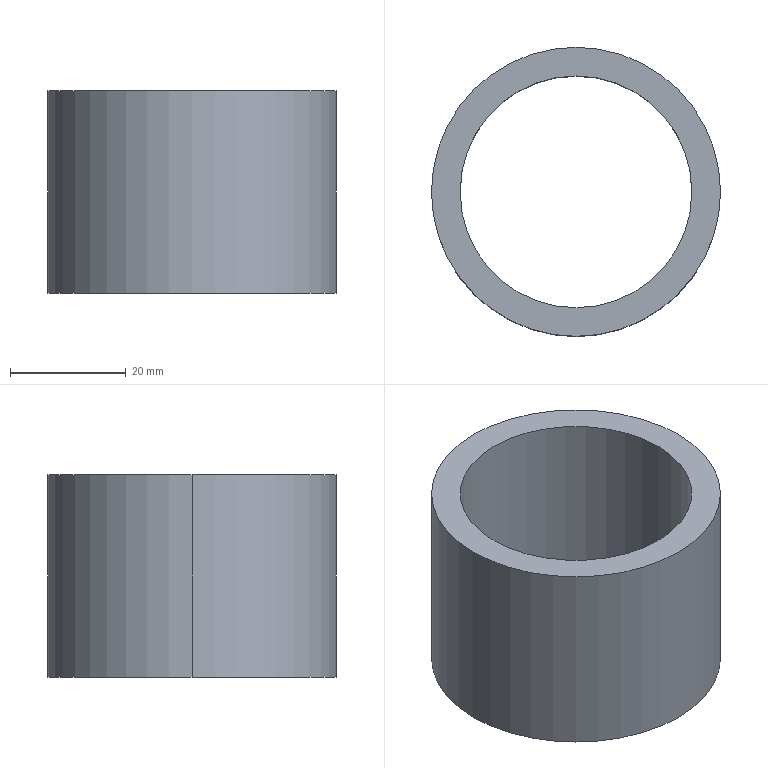Part | STEP file | LM-05-1226_default | 1 solid | 6 faces | box 50 x 50 x 35 mm | volume 24520 mm3 | cylinder 4 | plane 2 | commonest cylinder face diameters 40.1 x2 50 x2
STEP:
#1=CARTESIAN_POINT('',(0.,0.,0.));
#2=DIRECTION('',(0.,0.,1.));
#3=DIRECTION('',(1.,0.,0.));
#4=AXIS2_PLACEMENT_3D('',#1,#2,#3);
#5=CARTESIAN_POINT('',(-20.05,0.,17.5));
#6=VERTEX_POINT('',#5);
#7=CARTESIAN_POINT('',(-20.05,0.,-17.5));
#8=VERTEX_POINT('',#7);
#9=CARTESIAN_POINT('',(-20.05,0.,17.5));
#10=DIRECTION('',(0.,0.,-1.));
#11=VECTOR('',#10,1.);
#12=LINE('',#9,#11);
#13=CARTESIAN_POINT('',(0.,0.,17.5));
#14=DIRECTION('',(0.,0.,-1.));
#15=DIRECTION('',(-1.,0.,0.));
#16=AXIS2_PLACEMENT_3D('',#13,#14,#15);
#17=CYLINDRICAL_SURFACE('',#16,20.05);
#18=CARTESIAN_POINT('',(6.283,0.));
#19=DIRECTION('',(0.,1.));
#20=VECTOR('',#19,1.);
#21=LINE('',#18,#20);
#22=(GEOMETRIC_REPRESENTATION_CONTEXT(2)PARAMETRIC_REPRESENTATION_CONTEXT()REPRESENTATION_CONTEXT('',''));
#23=DEFINITIONAL_REPRESENTATION('',(#21),#22);
#24=PCURVE('',#17,#23);
#25=CARTESIAN_POINT('',(0.,0.,17.5));
#26=DIRECTION('',(0.,0.,-1.));
#27=DIRECTION('',(-1.,0.,0.));
#28=AXIS2_PLACEMENT_3D('',#25,#26,#27);
#29=CYLINDRICAL_SURFACE('',#28,20.05);
#30=CARTESIAN_POINT('',(0.,0.));
#31=DIRECTION('',(0.,1.));
#32=VECTOR('',#31,1.);
#33=LINE('',#30,#32);
#34=(GEOMETRIC_REPRESENTATION_CONTEXT(2)PARAMETRIC_REPRESENTATION_CONTEXT()REPRESENTATION_CONTEXT('',''));
#35=DEFINITIONAL_REPRESENTATION('',(#33),#34);
#36=PCURVE('',#29,#35);
#37=SURFACE_CURVE('',#12,(#24,#36),.PCURVE_S1.);
#38=EDGE_CURVE('',#6,#8,#37,.T.);
#39=ORIENTED_EDGE('',*,*,#38,.T.);
#40=CARTESIAN_POINT('',(20.05,0.,-17.5));
#41=VERTEX_POINT('',#40);
#42=CARTESIAN_POINT('',(0.,0.,-17.5));
#43=DIRECTION('',(0.,0.,1.));
#44=DIRECTION('',(1.,0.,0.));
#45=AXIS2_PLACEMENT_3D('',#42,#43,#44);
#46=CIRCLE('',#45,20.05);
#47=CARTESIAN_POINT('',(9.425,35.));
#48=DIRECTION('',(-1.,0.));
#49=VECTOR('',#48,1.);
#50=LINE('',#47,#49);
#51=(GEOMETRIC_REPRESENTATION_CONTEXT(2)PARAMETRIC_REPRESENTATION_CONTEXT()REPRESENTATION_CONTEXT('',''));
#52=DEFINITIONAL_REPRESENTATION('',(#50),#51);
#53=PCURVE('',#17,#52);
#54=CARTESIAN_POINT('',(0.,0.,-17.5));
#55=DIRECTION('',(0.,0.,1.));
#56=DIRECTION('',(1.,0.,0.));
#57=AXIS2_PLACEMENT_3D('',#54,#55,#56);
#58=PLANE('',#57);
#59=CARTESIAN_POINT('',(0.,0.));
#60=DIRECTION('',(1.,0.));
#61=AXIS2_PLACEMENT_2D('',#59,#60);
#62=CIRCLE('',#61,20.05);
#63=(GEOMETRIC_REPRESENTATION_CONTEXT(2)PARAMETRIC_REPRESENTATION_CONTEXT()REPRESENTATION_CONTEXT('',''));
#64=DEFINITIONAL_REPRESENTATION('',(#62),#63);
#65=PCURVE('',#58,#64);
#66=SURFACE_CURVE('',#46,(#53,#65),.PCURVE_S1.);
#67=EDGE_CURVE('',#8,#41,#66,.T.);
#68=ORIENTED_EDGE('',*,*,#67,.T.);
#69=CARTESIAN_POINT('',(20.05,0.,17.5));
#70=VERTEX_POINT('',#69);
#71=CARTESIAN_POINT('',(20.05,0.,17.5));
#72=DIRECTION('',(0.,0.,-1.));
#73=VECTOR('',#72,1.);
#74=LINE('',#71,#73);
#75=CARTESIAN_POINT('',(3.142,0.));
#76=DIRECTION('',(0.,1.));
#77=VECTOR('',#76,1.);
#78=LINE('',#75,#77);
#79=(GEOMETRIC_REPRESENTATION_CONTEXT(2)PARAMETRIC_REPRESENTATION_CONTEXT()REPRESENTATION_CONTEXT('',''));
#80=DEFINITIONAL_REPRESENTATION('',(#78),#79);
#81=PCURVE('',#17,#80);
#82=CARTESIAN_POINT('',(3.142,0.));
#83=DIRECTION('',(0.,1.));
#84=VECTOR('',#83,1.);
#85=LINE('',#82,#84);
#86=(GEOMETRIC_REPRESENTATION_CONTEXT(2)PARAMETRIC_REPRESENTATION_CONTEXT()REPRESENTATION_CONTEXT('',''));
#87=DEFINITIONAL_REPRESENTATION('',(#85),#86);
#88=PCURVE('',#29,#87);
#89=SURFACE_CURVE('',#74,(#81,#88),.PCURVE_S1.);
#90=EDGE_CURVE('',#70,#41,#89,.T.);
#91=ORIENTED_EDGE('',*,*,#90,.F.);
#92=CARTESIAN_POINT('',(0.,0.,17.5));
#93=DIRECTION('',(0.,0.,1.));
#94=DIRECTION('',(1.,0.,0.));
#95=AXIS2_PLACEMENT_3D('',#92,#93,#94);
#96=CIRCLE('',#95,20.05);
#97=CARTESIAN_POINT('',(9.425,0.));
#98=DIRECTION('',(-1.,0.));
#99=VECTOR('',#98,1.);
#100=LINE('',#97,#99);
#101=(GEOMETRIC_REPRESENTATION_CONTEXT(2)PARAMETRIC_REPRESENTATION_CONTEXT()REPRESENTATION_CONTEXT('',''));
#102=DEFINITIONAL_REPRESENTATION('',(#100),#101);
#103=PCURVE('',#17,#102);
#104=CARTESIAN_POINT('',(0.,0.,17.5));
#105=DIRECTION('',(0.,0.,1.));
#106=DIRECTION('',(1.,0.,0.));
#107=AXIS2_PLACEMENT_3D('',#104,#105,#106);
#108=PLANE('',#107);
#109=CARTESIAN_POINT('',(0.,0.));
#110=DIRECTION('',(1.,0.));
#111=AXIS2_PLACEMENT_2D('',#109,#110);
#112=CIRCLE('',#111,20.05);
#113=(GEOMETRIC_REPRESENTATION_CONTEXT(2)PARAMETRIC_REPRESENTATION_CONTEXT()REPRESENTATION_CONTEXT('',''));
#114=DEFINITIONAL_REPRESENTATION('',(#112),#113);
#115=PCURVE('',#108,#114);
#116=SURFACE_CURVE('',#96,(#103,#115),.PCURVE_S1.);
#117=EDGE_CURVE('',#6,#70,#116,.T.);
#118=ORIENTED_EDGE('',*,*,#117,.F.);
#119=EDGE_LOOP('',(#39,#68,#91,#118));
#120=FACE_BOUND('',#119,.F.);
#121=ADVANCED_FACE('',(#120),#17,.F.);
#122=CARTESIAN_POINT('',(25.,0.,17.5));
#123=VERTEX_POINT('',#122);
#124=CARTESIAN_POINT('',(-25.,0.,17.5));
#125=VERTEX_POINT('',#124);
#126=CARTESIAN_POINT('',(0.,0.,17.5));
#127=DIRECTION('',(0.,0.,1.));
#128=DIRECTION('',(1.,0.,0.));
#129=AXIS2_PLACEMENT_3D('',#126,#127,#128);
#130=CIRCLE('',#129,25.);
#131=CARTESIAN_POINT('',(0.,0.,17.5));
#132=DIRECTION('',(0.,0.,-1.));
#133=DIRECTION('',(-1.,0.,0.));
#134=AXIS2_PLACEMENT_3D('',#131,#132,#133);
#135=CYLINDRICAL_SURFACE('',#134,25.);
#136=CARTESIAN_POINT('',(3.142,0.));
#137=DIRECTION('',(-1.,0.));
#138=VECTOR('',#137,1.);
#139=LINE('',#136,#138);
#140=(GEOMETRIC_REPRESENTATION_CONTEXT(2)PARAMETRIC_REPRESENTATION_CONTEXT()REPRESENTATION_CONTEXT('',''));
#141=DEFINITIONAL_REPRESENTATION('',(#139),#140);
#142=PCURVE('',#135,#141);
#143=CARTESIAN_POINT('',(0.,0.));
#144=DIRECTION('',(1.,0.));
#145=AXIS2_PLACEMENT_2D('',#143,#144);
#146=CIRCLE('',#145,25.);
#147=(GEOMETRIC_REPRESENTATION_CONTEXT(2)PARAMETRIC_REPRESENTATION_CONTEXT()REPRESENTATION_CONTEXT('',''));
#148=DEFINITIONAL_REPRESENTATION('',(#146),#147);
#149=PCURVE('',#108,#148);
#150=SURFACE_CURVE('',#130,(#142,#149),.PCURVE_S1.);
#151=EDGE_CURVE('',#123,#125,#150,.T.);
#152=ORIENTED_EDGE('',*,*,#151,.F.);
#153=CARTESIAN_POINT('',(25.,0.,-17.5));
#154=VERTEX_POINT('',#153);
#155=CARTESIAN_POINT('',(25.,0.,17.5));
#156=DIRECTION('',(0.,0.,-1.));
#157=VECTOR('',#156,1.);
#158=LINE('',#155,#157);
#159=CARTESIAN_POINT('',(3.142,0.));
#160=DIRECTION('',(0.,1.));
#161=VECTOR('',#160,1.);
#162=LINE('',#159,#161);
#163=(GEOMETRIC_REPRESENTATION_CONTEXT(2)PARAMETRIC_REPRESENTATION_CONTEXT()REPRESENTATION_CONTEXT('',''));
#164=DEFINITIONAL_REPRESENTATION('',(#162),#163);
#165=PCURVE('',#135,#164);
#166=CARTESIAN_POINT('',(0.,0.,17.5));
#167=DIRECTION('',(0.,0.,-1.));
#168=DIRECTION('',(-1.,0.,0.));
#169=AXIS2_PLACEMENT_3D('',#166,#167,#168);
#170=CYLINDRICAL_SURFACE('',#169,25.);
#171=CARTESIAN_POINT('',(3.142,0.));
#172=DIRECTION('',(0.,1.));
#173=VECTOR('',#172,1.);
#174=LINE('',#171,#173);
#175=(GEOMETRIC_REPRESENTATION_CONTEXT(2)PARAMETRIC_REPRESENTATION_CONTEXT()REPRESENTATION_CONTEXT('',''));
#176=DEFINITIONAL_REPRESENTATION('',(#174),#175);
#177=PCURVE('',#170,#176);
#178=SURFACE_CURVE('',#158,(#165,#177),.PCURVE_S1.);
#179=EDGE_CURVE('',#123,#154,#178,.T.);
#180=ORIENTED_EDGE('',*,*,#179,.T.);
#181=CARTESIAN_POINT('',(-25.,0.,-17.5));
#182=VERTEX_POINT('',#181);
#183=CARTESIAN_POINT('',(0.,0.,-17.5));
#184=DIRECTION('',(0.,0.,1.));
#185=DIRECTION('',(1.,0.,0.));
#186=AXIS2_PLACEMENT_3D('',#183,#184,#185);
#187=CIRCLE('',#186,25.);
#188=CARTESIAN_POINT('',(3.142,35.));
#189=DIRECTION('',(-1.,0.));
#190=VECTOR('',#189,1.);
#191=LINE('',#188,#190);
#192=(GEOMETRIC_REPRESENTATION_CONTEXT(2)PARAMETRIC_REPRESENTATION_CONTEXT()REPRESENTATION_CONTEXT('',''));
#193=DEFINITIONAL_REPRESENTATION('',(#191),#192);
#194=PCURVE('',#135,#193);
#195=CARTESIAN_POINT('',(0.,0.));
#196=DIRECTION('',(1.,0.));
#197=AXIS2_PLACEMENT_2D('',#195,#196);
#198=CIRCLE('',#197,25.);
#199=(GEOMETRIC_REPRESENTATION_CONTEXT(2)PARAMETRIC_REPRESENTATION_CONTEXT()REPRESENTATION_CONTEXT('',''));
#200=DEFINITIONAL_REPRESENTATION('',(#198),#199);
#201=PCURVE('',#58,#200);
#202=SURFACE_CURVE('',#187,(#194,#201),.PCURVE_S1.);
#203=EDGE_CURVE('',#154,#182,#202,.T.);
#204=ORIENTED_EDGE('',*,*,#203,.T.);
#205=CARTESIAN_POINT('',(-25.,0.,17.5));
#206=DIRECTION('',(0.,0.,-1.));
#207=VECTOR('',#206,1.);
#208=LINE('',#205,#207);
#209=CARTESIAN_POINT('',(0.,0.));
#210=DIRECTION('',(0.,1.));
#211=VECTOR('',#210,1.);
#212=LINE('',#209,#211);
#213=(GEOMETRIC_REPRESENTATION_CONTEXT(2)PARAMETRIC_REPRESENTATION_CONTEXT()REPRESENTATION_CONTEXT('',''));
#214=DEFINITIONAL_REPRESENTATION('',(#212),#213);
#215=PCURVE('',#135,#214);
#216=CARTESIAN_POINT('',(6.283,0.));
#217=DIRECTION('',(0.,1.));
#218=VECTOR('',#217,1.);
#219=LINE('',#216,#218);
#220=(GEOMETRIC_REPRESENTATION_CONTEXT(2)PARAMETRIC_REPRESENTATION_CONTEXT()REPRESENTATION_CONTEXT('',''));
#221=DEFINITIONAL_REPRESENTATION('',(#219),#220);
#222=PCURVE('',#170,#221);
#223=SURFACE_CURVE('',#208,(#215,#222),.PCURVE_S1.);
#224=EDGE_CURVE('',#125,#182,#223,.T.);
#225=ORIENTED_EDGE('',*,*,#224,.F.);
#226=EDGE_LOOP('',(#152,#180,#204,#225));
#227=FACE_BOUND('',#226,.T.);
#228=ADVANCED_FACE('',(#227),#135,.T.);
#229=CARTESIAN_POINT('',(0.,0.,17.5));
#230=DIRECTION('',(0.,0.,1.));
#231=DIRECTION('',(1.,0.,0.));
#232=AXIS2_PLACEMENT_3D('',#229,#230,#231);
#233=CIRCLE('',#232,25.);
#234=CARTESIAN_POINT('',(0.,0.));
#235=DIRECTION('',(1.,0.));
#236=AXIS2_PLACEMENT_2D('',#234,#235);
#237=CIRCLE('',#236,25.);
#238=(GEOMETRIC_REPRESENTATION_CONTEXT(2)PARAMETRIC_REPRESENTATION_CONTEXT()REPRESENTATION_CONTEXT('',''));
#239=DEFINITIONAL_REPRESENTATION('',(#237),#238);
#240=PCURVE('',#108,#239);
#241=CARTESIAN_POINT('',(9.425,0.));
#242=DIRECTION('',(-1.,0.));
#243=VECTOR('',#242,1.);
#244=LINE('',#241,#243);
#245=(GEOMETRIC_REPRESENTATION_CONTEXT(2)PARAMETRIC_REPRESENTATION_CONTEXT()REPRESENTATION_CONTEXT('',''));
#246=DEFINITIONAL_REPRESENTATION('',(#244),#245);
#247=PCURVE('',#170,#246);
#248=SURFACE_CURVE('',#233,(#240,#247),.PCURVE_S1.);
#249=EDGE_CURVE('',#125,#123,#248,.T.);
#250=ORIENTED_EDGE('',*,*,#249,.T.);
#251=ORIENTED_EDGE('',*,*,#151,.T.);
#252=EDGE_LOOP('',(#250,#251));
#253=FACE_BOUND('',#252,.T.);
#254=ORIENTED_EDGE('',*,*,#117,.F.);
#255=CARTESIAN_POINT('',(0.,0.,17.5));
#256=DIRECTION('',(0.,0.,1.));
#257=DIRECTION('',(1.,0.,0.));
#258=AXIS2_PLACEMENT_3D('',#255,#256,#257);
#259=CIRCLE('',#258,20.05);
#260=CARTESIAN_POINT('',(0.,0.));
#261=DIRECTION('',(1.,0.));
#262=AXIS2_PLACEMENT_2D('',#260,#261);
#263=CIRCLE('',#262,20.05);
#264=(GEOMETRIC_REPRESENTATION_CONTEXT(2)PARAMETRIC_REPRESENTATION_CONTEXT()REPRESENTATION_CONTEXT('',''));
#265=DEFINITIONAL_REPRESENTATION('',(#263),#264);
#266=PCURVE('',#108,#265);
#267=CARTESIAN_POINT('',(3.142,0.));
#268=DIRECTION('',(-1.,0.));
#269=VECTOR('',#268,1.);
#270=LINE('',#267,#269);
#271=(GEOMETRIC_REPRESENTATION_CONTEXT(2)PARAMETRIC_REPRESENTATION_CONTEXT()REPRESENTATION_CONTEXT('',''));
#272=DEFINITIONAL_REPRESENTATION('',(#270),#271);
#273=PCURVE('',#29,#272);
#274=SURFACE_CURVE('',#259,(#266,#273),.PCURVE_S1.);
#275=EDGE_CURVE('',#70,#6,#274,.T.);
#276=ORIENTED_EDGE('',*,*,#275,.F.);
#277=EDGE_LOOP('',(#254,#276));
#278=FACE_BOUND('',#277,.T.);
#279=ADVANCED_FACE('',(#253,#278),#108,.T.);
#280=CARTESIAN_POINT('',(0.,0.,-17.5));
#281=DIRECTION('',(0.,0.,1.));
#282=DIRECTION('',(1.,0.,0.));
#283=AXIS2_PLACEMENT_3D('',#280,#281,#282);
#284=CIRCLE('',#283,25.);
#285=CARTESIAN_POINT('',(0.,0.));
#286=DIRECTION('',(1.,0.));
#287=AXIS2_PLACEMENT_2D('',#285,#286);
#288=CIRCLE('',#287,25.);
#289=(GEOMETRIC_REPRESENTATION_CONTEXT(2)PARAMETRIC_REPRESENTATION_CONTEXT()REPRESENTATION_CONTEXT('',''));
#290=DEFINITIONAL_REPRESENTATION('',(#288),#289);
#291=PCURVE('',#58,#290);
#292=CARTESIAN_POINT('',(9.425,35.));
#293=DIRECTION('',(-1.,0.));
#294=VECTOR('',#293,1.);
#295=LINE('',#292,#294);
#296=(GEOMETRIC_REPRESENTATION_CONTEXT(2)PARAMETRIC_REPRESENTATION_CONTEXT()REPRESENTATION_CONTEXT('',''));
#297=DEFINITIONAL_REPRESENTATION('',(#295),#296);
#298=PCURVE('',#170,#297);
#299=SURFACE_CURVE('',#284,(#291,#298),.PCURVE_S1.);
#300=EDGE_CURVE('',#182,#154,#299,.T.);
#301=ORIENTED_EDGE('',*,*,#300,.F.);
#302=ORIENTED_EDGE('',*,*,#203,.F.);
#303=EDGE_LOOP('',(#301,#302));
#304=FACE_BOUND('',#303,.T.);
#305=ORIENTED_EDGE('',*,*,#67,.T.);
#306=CARTESIAN_POINT('',(0.,0.,-17.5));
#307=DIRECTION('',(0.,0.,1.));
#308=DIRECTION('',(1.,0.,0.));
#309=AXIS2_PLACEMENT_3D('',#306,#307,#308);
#310=CIRCLE('',#309,20.05);
#311=CARTESIAN_POINT('',(0.,0.));
#312=DIRECTION('',(1.,0.));
#313=AXIS2_PLACEMENT_2D('',#311,#312);
#314=CIRCLE('',#313,20.05);
#315=(GEOMETRIC_REPRESENTATION_CONTEXT(2)PARAMETRIC_REPRESENTATION_CONTEXT()REPRESENTATION_CONTEXT('',''));
#316=DEFINITIONAL_REPRESENTATION('',(#314),#315);
#317=PCURVE('',#58,#316);
#318=CARTESIAN_POINT('',(3.142,35.));
#319=DIRECTION('',(-1.,0.));
#320=VECTOR('',#319,1.);
#321=LINE('',#318,#320);
#322=(GEOMETRIC_REPRESENTATION_CONTEXT(2)PARAMETRIC_REPRESENTATION_CONTEXT()REPRESENTATION_CONTEXT('',''));
#323=DEFINITIONAL_REPRESENTATION('',(#321),#322);
#324=PCURVE('',#29,#323);
#325=SURFACE_CURVE('',#310,(#317,#324),.PCURVE_S1.);
#326=EDGE_CURVE('',#41,#8,#325,.T.);
#327=ORIENTED_EDGE('',*,*,#326,.T.);
#328=EDGE_LOOP('',(#305,#327));
#329=FACE_BOUND('',#328,.T.);
#330=ADVANCED_FACE('',(#304,#329),#58,.F.);
#331=ORIENTED_EDGE('',*,*,#179,.F.);
#332=ORIENTED_EDGE('',*,*,#249,.F.);
#333=ORIENTED_EDGE('',*,*,#224,.T.);
#334=ORIENTED_EDGE('',*,*,#300,.T.);
#335=EDGE_LOOP('',(#331,#332,#333,#334));
#336=FACE_BOUND('',#335,.T.);
#337=ADVANCED_FACE('',(#336),#170,.T.);
#338=ORIENTED_EDGE('',*,*,#326,.T.);
#339=ORIENTED_EDGE('',*,*,#38,.F.);
#340=ORIENTED_EDGE('',*,*,#275,.F.);
#341=ORIENTED_EDGE('',*,*,#90,.T.);
#342=EDGE_LOOP('',(#338,#339,#340,#341));
#343=FACE_BOUND('',#342,.F.);
#344=ADVANCED_FACE('',(#343),#29,.F.);
#345=CLOSED_SHELL('',(#121,#228,#279,#330,#337,#344));
#346=MANIFOLD_SOLID_BREP('',#345);
#347=(LENGTH_UNIT()NAMED_UNIT(*)SI_UNIT(.MILLI.,.METRE.));
#348=UNCERTAINTY_MEASURE_WITH_UNIT(LENGTH_MEASURE(0.0000001),#347,'','');
#349=(NAMED_UNIT(*)PLANE_ANGLE_UNIT()SI_UNIT($,.RADIAN.));
#350=(NAMED_UNIT(*)SI_UNIT($,.STERADIAN.)SOLID_ANGLE_UNIT());
#351=(GEOMETRIC_REPRESENTATION_CONTEXT(3)GLOBAL_UNCERTAINTY_ASSIGNED_CONTEXT((#348))GLOBAL_UNIT_ASSIGNED_CONTEXT((#347,#349,#350))REPRESENTATION_CONTEXT('',''));
#352=ADVANCED_BREP_SHAPE_REPRESENTATION('',(#4,#346),#351);